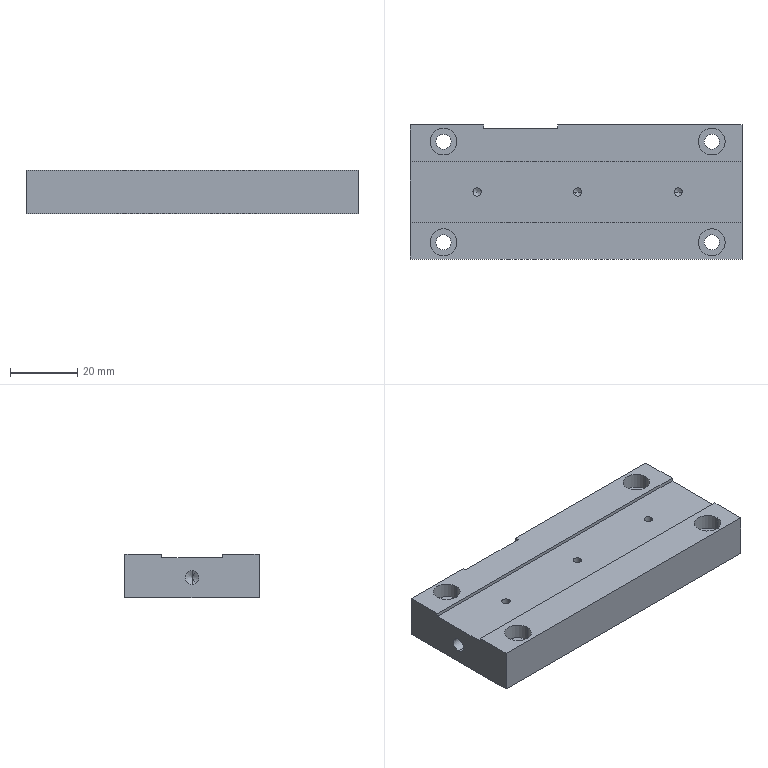Part | STEP file | PN_0006 Mount electronic clip pad block 3 | 1 solid | 66 faces | box 99 x 40 x 13 mm | volume 46951 mm3 | cylinder 32 | plane 18 | cone 16 | commonest cylinder face diameters 4.5 x8 8 x8 2.5 x6 4.2 x6 3.3 x4